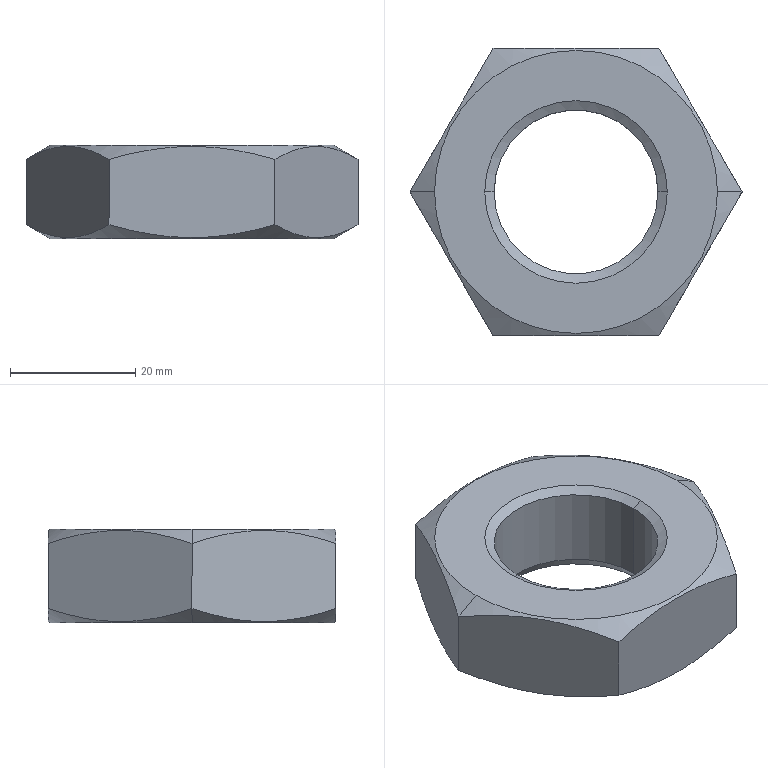Part | SolidWorks | features RevCut 2, Chamfer 1, Extrusion 1, LPattern 1 | 1 solid | 18 faces | box 53.116 x 46 x 15 mm | volume 18987 mm3 | cone 8 | plane 8 | cylinder 2 | commonest cylinder face diameters 26.211 x2
STEP:
#1=CARTESIAN_POINT('',(-13.106,0.,-0.866));
#2=VERTEX_POINT('',#1);
#3=CARTESIAN_POINT('',(13.106,0.,-0.866));
#4=VERTEX_POINT('',#3);
#5=CARTESIAN_POINT('',(0.,0.,-0.866));
#6=DIRECTION('',(0.,0.,1.));
#7=DIRECTION('',(1.,0.,0.));
#8=AXIS2_PLACEMENT_3D('',#5,#6,#7);
#9=CIRCLE('',#8,13.106);
#10=EDGE_CURVE('',#2,#4,#9,.T.);
#11=ORIENTED_EDGE('',*,*,#10,.F.);
#12=CARTESIAN_POINT('',(-14.606,0.,0.));
#13=VERTEX_POINT('',#12);
#14=CARTESIAN_POINT('',(-13.106,0.,-0.866));
#15=DIRECTION('',(-0.866,0.,0.5));
#16=VECTOR('',#15,1000.);
#17=LINE('',#14,#16);
#18=EDGE_CURVE('',#2,#13,#17,.T.);
#19=ORIENTED_EDGE('',*,*,#18,.T.);
#20=CARTESIAN_POINT('',(14.606,0.,0.));
#21=VERTEX_POINT('',#20);
#22=CARTESIAN_POINT('',(0.,0.,0.));
#23=DIRECTION('',(0.,0.,-1.));
#24=DIRECTION('',(1.,0.,0.));
#25=AXIS2_PLACEMENT_3D('',#22,#23,#24);
#26=CIRCLE('',#25,14.606);
#27=EDGE_CURVE('',#21,#13,#26,.T.);
#28=ORIENTED_EDGE('',*,*,#27,.F.);
#29=CARTESIAN_POINT('',(13.106,0.,-0.866));
#30=DIRECTION('',(0.866,0.,0.5));
#31=VECTOR('',#30,1000.);
#32=LINE('',#29,#31);
#33=EDGE_CURVE('',#4,#21,#32,.T.);
#34=ORIENTED_EDGE('',*,*,#33,.F.);
#35=EDGE_LOOP('',(#11,#19,#28,#34));
#36=FACE_OUTER_BOUND('',#35,.T.);
#37=CARTESIAN_POINT('',(0.,0.,-0.866));
#38=DIRECTION('',(0.,0.,1.));
#39=DIRECTION('',(1.,0.,0.));
#40=AXIS2_PLACEMENT_3D('',#37,#38,#39);
#41=CONICAL_SURFACE('',#40,13.106,1.047);
#42=ADVANCED_FACE('',(#36),#41,.F.);
#43=CARTESIAN_POINT('',(13.106,0.,-13.5));
#44=VERTEX_POINT('',#43);
#45=CARTESIAN_POINT('',(-13.106,0.,-13.5));
#46=VERTEX_POINT('',#45);
#47=CARTESIAN_POINT('',(0.,0.,-13.5));
#48=DIRECTION('',(0.,0.,-1.));
#49=DIRECTION('',(1.,0.,0.));
#50=AXIS2_PLACEMENT_3D('',#47,#48,#49);
#51=CIRCLE('',#50,13.106);
#52=EDGE_CURVE('',#44,#46,#51,.T.);
#53=ORIENTED_EDGE('',*,*,#52,.F.);
#54=CARTESIAN_POINT('',(13.972,0.,-15.));
#55=VERTEX_POINT('',#54);
#56=CARTESIAN_POINT('',(13.972,0.,-15.));
#57=DIRECTION('',(0.5,0.,-0.866));
#58=VECTOR('',#57,1000.);
#59=LINE('',#56,#58);
#60=EDGE_CURVE('',#44,#55,#59,.T.);
#61=ORIENTED_EDGE('',*,*,#60,.T.);
#62=CARTESIAN_POINT('',(-13.972,0.,-15.));
#63=VERTEX_POINT('',#62);
#64=CARTESIAN_POINT('',(0.,0.,-15.));
#65=DIRECTION('',(0.,0.,1.));
#66=DIRECTION('',(1.,0.,0.));
#67=AXIS2_PLACEMENT_3D('',#64,#65,#66);
#68=CIRCLE('',#67,13.972);
#69=EDGE_CURVE('',#63,#55,#68,.T.);
#70=ORIENTED_EDGE('',*,*,#69,.F.);
#71=CARTESIAN_POINT('',(-13.972,0.,-15.));
#72=DIRECTION('',(-0.5,0.,-0.866));
#73=VECTOR('',#72,1000.);
#74=LINE('',#71,#73);
#75=EDGE_CURVE('',#46,#63,#74,.T.);
#76=ORIENTED_EDGE('',*,*,#75,.F.);
#77=EDGE_LOOP('',(#53,#61,#70,#76));
#78=FACE_OUTER_BOUND('',#77,.T.);
#79=CARTESIAN_POINT('',(0.,0.,-15.));
#80=DIRECTION('',(0.,0.,-1.));
#81=DIRECTION('',(-1.,0.,0.));
#82=AXIS2_PLACEMENT_3D('',#79,#80,#81);
#83=CONICAL_SURFACE('',#82,13.972,0.5236);
#84=ADVANCED_FACE('',(#78),#83,.F.);
#85=CARTESIAN_POINT('',(-22.625,0.,0.));
#86=VERTEX_POINT('',#85);
#87=CARTESIAN_POINT('',(22.625,0.,0.));
#88=VERTEX_POINT('',#87);
#89=CARTESIAN_POINT('',(0.,0.,0.));
#90=DIRECTION('',(0.,0.,-1.));
#91=DIRECTION('',(-1.,0.,0.));
#92=AXIS2_PLACEMENT_3D('',#89,#90,#91);
#93=CIRCLE('',#92,22.625);
#94=EDGE_CURVE('',#86,#88,#93,.T.);
#95=ORIENTED_EDGE('',*,*,#94,.T.);
#96=CARTESIAN_POINT('',(26.558,0.,-2.271));
#97=VERTEX_POINT('',#96);
#98=CARTESIAN_POINT('',(22.625,0.,0.));
#99=DIRECTION('',(0.866,0.,-0.5));
#100=VECTOR('',#99,1000.);
#101=LINE('',#98,#100);
#102=EDGE_CURVE('',#88,#97,#101,.T.);
#103=ORIENTED_EDGE('',*,*,#102,.T.);
#104=CARTESIAN_POINT('',(13.279,23.,-2.271));
#105=VERTEX_POINT('',#104);
#106=CARTESIAN_POINT('',(26.558,0.,-2.271));
#107=CARTESIAN_POINT('',(25.474,1.878,-1.645));
#108=CARTESIAN_POINT('',(24.382,3.769,-1.129));
#109=CARTESIAN_POINT('',(22.175,7.591,-0.4144));
#110=CARTESIAN_POINT('',(21.06,9.523,-0.218));
#111=CARTESIAN_POINT('',(19.649,11.967,-0.2162));
#112=CARTESIAN_POINT('',(19.365,12.458,-0.2279));
#113=CARTESIAN_POINT('',(18.801,13.436,-0.2751));
#114=CARTESIAN_POINT('',(18.519,13.924,-0.3106));
#115=CARTESIAN_POINT('',(17.678,15.381,-0.4511));
#116=CARTESIAN_POINT('',(17.121,16.346,-0.5901));
#117=CARTESIAN_POINT('',(15.459,19.224,-1.127));
#118=CARTESIAN_POINT('',(14.365,21.12,-1.644));
#119=CARTESIAN_POINT('',(13.279,23.,-2.271));
#120=B_SPLINE_CURVE_WITH_KNOTS('',3,(#106,#107,#108,#109,#110,#111,#112,#113,#114,#115,#116,#117,#118,#119),.UNSPECIFIED.,.F.,.F.,(4,2,2,2,2,2,4),(0.000000238,0.006706,0.01341,0.01509,0.01676,0.02012,0.02682),.UNSPECIFIED.);
#121=EDGE_CURVE('',#97,#105,#120,.T.);
#122=ORIENTED_EDGE('',*,*,#121,.T.);
#123=CARTESIAN_POINT('',(-13.279,23.,-2.271));
#124=VERTEX_POINT('',#123);
#125=CARTESIAN_POINT('',(13.279,23.,-2.271));
#126=CARTESIAN_POINT('',(11.133,23.,-1.651));
#127=CARTESIAN_POINT('',(8.958,23.,-1.135));
#128=CARTESIAN_POINT('',(5.632,23.,-0.595));
#129=CARTESIAN_POINT('',(4.511,23.,-0.4541));
#130=CARTESIAN_POINT('',(2.252,23.,-0.2644));
#131=CARTESIAN_POINT('',(1.126,23.,-0.2166));
#132=CARTESIAN_POINT('',(-2.241,23.,-0.2163));
#133=CARTESIAN_POINT('',(-4.471,23.,-0.409));
#134=CARTESIAN_POINT('',(-7.797,23.,-0.9453));
#135=CARTESIAN_POINT('',(-8.904,23.,-1.165));
#136=CARTESIAN_POINT('',(-11.109,23.,-1.673));
#137=CARTESIAN_POINT('',(-12.199,23.,-1.959));
#138=CARTESIAN_POINT('',(-13.279,23.,-2.271));
#139=B_SPLINE_CURVE_WITH_KNOTS('',3,(#125,#126,#127,#128,#129,#130,#131,#132,#133,#134,#135,#136,#137,#138),.UNSPECIFIED.,.F.,.F.,(4,2,2,2,2,2,4),(0.00977,0.01647,0.01982,0.02317,0.02987,0.03323,0.03658),.UNSPECIFIED.);
#140=EDGE_CURVE('',#105,#124,#139,.T.);
#141=ORIENTED_EDGE('',*,*,#140,.T.);
#142=CARTESIAN_POINT('',(-26.558,0.,-2.271));
#143=VERTEX_POINT('',#142);
#144=CARTESIAN_POINT('',(-13.279,23.,-2.271));
#145=CARTESIAN_POINT('',(-14.363,21.122,-1.645));
#146=CARTESIAN_POINT('',(-15.455,19.231,-1.129));
#147=CARTESIAN_POINT('',(-17.662,15.409,-0.4144));
#148=CARTESIAN_POINT('',(-18.777,13.477,-0.218));
#149=CARTESIAN_POINT('',(-20.188,11.033,-0.2162));
#150=CARTESIAN_POINT('',(-20.472,10.542,-0.2279));
#151=CARTESIAN_POINT('',(-21.037,9.564,-0.2751));
#152=CARTESIAN_POINT('',(-21.318,9.076,-0.3106));
#153=CARTESIAN_POINT('',(-22.159,7.619,-0.4511));
#154=CARTESIAN_POINT('',(-22.717,6.654,-0.5901));
#155=CARTESIAN_POINT('',(-24.378,3.776,-1.127));
#156=CARTESIAN_POINT('',(-25.473,1.88,-1.644));
#157=CARTESIAN_POINT('',(-26.558,0.,-2.271));
#158=B_SPLINE_CURVE_WITH_KNOTS('',3,(#144,#145,#146,#147,#148,#149,#150,#151,#152,#153,#154,#155,#156,#157),.UNSPECIFIED.,.F.,.F.,(4,2,2,2,2,2,4),(0.000000238,0.006706,0.01341,0.01509,0.01676,0.02012,0.02682),.UNSPECIFIED.);
#159=EDGE_CURVE('',#124,#143,#158,.T.);
#160=ORIENTED_EDGE('',*,*,#159,.T.);
#161=CARTESIAN_POINT('',(-22.625,0.,0.));
#162=DIRECTION('',(-0.866,0.,-0.5));
#163=VECTOR('',#162,1000.);
#164=LINE('',#161,#163);
#165=EDGE_CURVE('',#86,#143,#164,.T.);
#166=ORIENTED_EDGE('',*,*,#165,.F.);
#167=EDGE_LOOP('',(#95,#103,#122,#141,#160,#166));
#168=FACE_OUTER_BOUND('',#167,.T.);
#169=CARTESIAN_POINT('',(0.,0.,0.));
#170=DIRECTION('',(0.,0.,-1.));
#171=DIRECTION('',(-1.,0.,0.));
#172=AXIS2_PLACEMENT_3D('',#169,#170,#171);
#173=CONICAL_SURFACE('',#172,22.625,1.047);
#174=ADVANCED_FACE('',(#168),#173,.T.);
#175=CARTESIAN_POINT('',(-22.625,0.,-15.));
#176=VERTEX_POINT('',#175);
#177=CARTESIAN_POINT('',(22.625,0.,-15.));
#178=VERTEX_POINT('',#177);
#179=CARTESIAN_POINT('',(0.,0.,-15.));
#180=DIRECTION('',(0.,0.,-1.));
#181=DIRECTION('',(-1.,0.,0.));
#182=AXIS2_PLACEMENT_3D('',#179,#180,#181);
#183=CIRCLE('',#182,22.625);
#184=EDGE_CURVE('',#176,#178,#183,.T.);
#185=ORIENTED_EDGE('',*,*,#184,.F.);
#186=CARTESIAN_POINT('',(-26.558,0.,-12.729));
#187=VERTEX_POINT('',#186);
#188=CARTESIAN_POINT('',(-26.558,0.,-12.729));
#189=DIRECTION('',(-0.866,0.,0.5));
#190=VECTOR('',#189,1000.);
#191=LINE('',#188,#190);
#192=EDGE_CURVE('',#176,#187,#191,.T.);
#193=ORIENTED_EDGE('',*,*,#192,.T.);
#194=CARTESIAN_POINT('',(-13.279,23.,-12.729));
#195=VERTEX_POINT('',#194);
#196=CARTESIAN_POINT('',(-26.558,0.,-12.729));
#197=CARTESIAN_POINT('',(-25.474,1.878,-13.355));
#198=CARTESIAN_POINT('',(-24.382,3.769,-13.871));
#199=CARTESIAN_POINT('',(-22.175,7.591,-14.586));
#200=CARTESIAN_POINT('',(-21.06,9.523,-14.782));
#201=CARTESIAN_POINT('',(-19.649,11.967,-14.784));
#202=CARTESIAN_POINT('',(-19.365,12.458,-14.772));
#203=CARTESIAN_POINT('',(-18.801,13.436,-14.725));
#204=CARTESIAN_POINT('',(-18.519,13.924,-14.689));
#205=CARTESIAN_POINT('',(-17.678,15.381,-14.549));
#206=CARTESIAN_POINT('',(-17.121,16.346,-14.41));
#207=CARTESIAN_POINT('',(-15.459,19.224,-13.873));
#208=CARTESIAN_POINT('',(-14.365,21.12,-13.356));
#209=CARTESIAN_POINT('',(-13.279,23.,-12.729));
#210=B_SPLINE_CURVE_WITH_KNOTS('',3,(#196,#197,#198,#199,#200,#201,#202,#203,#204,#205,#206,#207,#208,#209),.UNSPECIFIED.,.F.,.F.,(4,2,2,2,2,2,4),(0.000000238,0.006706,0.01341,0.01509,0.01676,0.02012,0.02682),.UNSPECIFIED.);
#211=EDGE_CURVE('',#187,#195,#210,.T.);
#212=ORIENTED_EDGE('',*,*,#211,.T.);
#213=CARTESIAN_POINT('',(13.279,23.,-12.729));
#214=VERTEX_POINT('',#213);
#215=CARTESIAN_POINT('',(-13.279,23.,-12.729));
#216=CARTESIAN_POINT('',(-12.199,23.,-13.041));
#217=CARTESIAN_POINT('',(-11.109,23.,-13.327));
#218=CARTESIAN_POINT('',(-8.904,23.,-13.835));
#219=CARTESIAN_POINT('',(-7.797,23.,-14.055));
#220=CARTESIAN_POINT('',(-4.471,23.,-14.591));
#221=CARTESIAN_POINT('',(-2.241,23.,-14.784));
#222=CARTESIAN_POINT('',(1.126,23.,-14.783));
#223=CARTESIAN_POINT('',(2.252,23.,-14.736));
#224=CARTESIAN_POINT('',(4.511,23.,-14.546));
#225=CARTESIAN_POINT('',(5.632,23.,-14.405));
#226=CARTESIAN_POINT('',(8.958,23.,-13.865));
#227=CARTESIAN_POINT('',(11.133,23.,-13.349));
#228=CARTESIAN_POINT('',(13.279,23.,-12.729));
#229=B_SPLINE_CURVE_WITH_KNOTS('',3,(#215,#216,#217,#218,#219,#220,#221,#222,#223,#224,#225,#226,#227,#228),.UNSPECIFIED.,.F.,.F.,(4,2,2,2,2,2,4),(0.02366,0.02702,0.03038,0.0371,0.04045,0.04381,0.05053),.UNSPECIFIED.);
#230=EDGE_CURVE('',#195,#214,#229,.T.);
#231=ORIENTED_EDGE('',*,*,#230,.T.);
#232=CARTESIAN_POINT('',(26.558,0.,-12.729));
#233=VERTEX_POINT('',#232);
#234=CARTESIAN_POINT('',(13.279,23.,-12.729));
#235=CARTESIAN_POINT('',(14.363,21.122,-13.355));
#236=CARTESIAN_POINT('',(15.455,19.231,-13.871));
#237=CARTESIAN_POINT('',(17.662,15.409,-14.586));
#238=CARTESIAN_POINT('',(18.777,13.477,-14.782));
#239=CARTESIAN_POINT('',(20.188,11.033,-14.784));
#240=CARTESIAN_POINT('',(20.472,10.542,-14.772));
#241=CARTESIAN_POINT('',(21.037,9.564,-14.725));
#242=CARTESIAN_POINT('',(21.318,9.076,-14.689));
#243=CARTESIAN_POINT('',(22.159,7.619,-14.549));
#244=CARTESIAN_POINT('',(22.717,6.654,-14.41));
#245=CARTESIAN_POINT('',(24.378,3.776,-13.873));
#246=CARTESIAN_POINT('',(25.473,1.88,-13.356));
#247=CARTESIAN_POINT('',(26.558,0.,-12.729));
#248=B_SPLINE_CURVE_WITH_KNOTS('',3,(#234,#235,#236,#237,#238,#239,#240,#241,#242,#243,#244,#245,#246,#247),.UNSPECIFIED.,.F.,.F.,(4,2,2,2,2,2,4),(0.000000238,0.006706,0.01341,0.01509,0.01676,0.02012,0.02682),.UNSPECIFIED.);
#249=EDGE_CURVE('',#214,#233,#248,.T.);
#250=ORIENTED_EDGE('',*,*,#249,.T.);
#251=CARTESIAN_POINT('',(26.558,0.,-12.729));
#252=DIRECTION('',(0.866,0.,0.5));
#253=VECTOR('',#252,1000.);
#254=LINE('',#251,#253);
#255=EDGE_CURVE('',#178,#233,#254,.T.);
#256=ORIENTED_EDGE('',*,*,#255,.F.);
#257=EDGE_LOOP('',(#185,#193,#212,#231,#250,#256));
#258=FACE_OUTER_BOUND('',#257,.T.);
#259=CARTESIAN_POINT('',(0.,0.,-12.729));
#260=DIRECTION('',(0.,0.,1.));
#261=DIRECTION('',(1.,0.,0.));
#262=AXIS2_PLACEMENT_3D('',#259,#260,#261);
#263=CONICAL_SURFACE('',#262,26.558,1.047);
#264=ADVANCED_FACE('',(#258),#263,.T.);
#265=ORIENTED_EDGE('',*,*,#52,.T.);
#266=CARTESIAN_POINT('',(-13.106,0.,-15.));
#267=DIRECTION('',(0.,0.,1.));
#268=VECTOR('',#267,1000.);
#269=LINE('',#266,#268);
#270=EDGE_CURVE('',#46,#2,#269,.T.);
#271=ORIENTED_EDGE('',*,*,#270,.T.);
#272=ORIENTED_EDGE('',*,*,#10,.T.);
#273=CARTESIAN_POINT('',(13.106,0.,-15.));
#274=DIRECTION('',(0.,0.,1.));
#275=VECTOR('',#274,1000.);
#276=LINE('',#273,#275);
#277=EDGE_CURVE('',#44,#4,#276,.T.);
#278=ORIENTED_EDGE('',*,*,#277,.F.);
#279=EDGE_LOOP('',(#265,#271,#272,#278));
#280=FACE_OUTER_BOUND('',#279,.T.);
#281=CARTESIAN_POINT('',(0.,0.,-15.));
#282=DIRECTION('',(0.,0.,1.));
#283=DIRECTION('',(1.,0.,0.));
#284=AXIS2_PLACEMENT_3D('',#281,#282,#283);
#285=CYLINDRICAL_SURFACE('',#284,13.106);
#286=ADVANCED_FACE('',(#280),#285,.F.);
#287=CARTESIAN_POINT('',(-13.279,-23.,-2.271));
#288=VERTEX_POINT('',#287);
#289=CARTESIAN_POINT('',(13.279,-23.,-2.271));
#290=VERTEX_POINT('',#289);
#291=CARTESIAN_POINT('',(-13.279,-23.,-2.271));
#292=CARTESIAN_POINT('',(-12.199,-23.,-1.959));
#293=CARTESIAN_POINT('',(-11.109,-23.,-1.673));
#294=CARTESIAN_POINT('',(-8.904,-23.,-1.165));
#295=CARTESIAN_POINT('',(-7.797,-23.,-0.9453));
#296=CARTESIAN_POINT('',(-4.471,-23.,-0.409));
#297=CARTESIAN_POINT('',(-2.241,-23.,-0.2163));
#298=CARTESIAN_POINT('',(1.126,-23.,-0.2166));
#299=CARTESIAN_POINT('',(2.252,-23.,-0.2644));
#300=CARTESIAN_POINT('',(4.511,-23.,-0.4541));
#301=CARTESIAN_POINT('',(5.632,-23.,-0.595));
#302=CARTESIAN_POINT('',(8.958,-23.,-1.135));
#303=CARTESIAN_POINT('',(11.133,-23.,-1.651));
#304=CARTESIAN_POINT('',(13.279,-23.,-2.271));
#305=B_SPLINE_CURVE_WITH_KNOTS('',3,(#291,#292,#293,#294,#295,#296,#297,#298,#299,#300,#301,#302,#303,#304),.UNSPECIFIED.,.F.,.F.,(4,2,2,2,2,2,4),(0.02366,0.02702,0.03038,0.0371,0.04045,0.04381,0.05053),.UNSPECIFIED.);
#306=EDGE_CURVE('',#288,#290,#305,.T.);
#307=ORIENTED_EDGE('',*,*,#306,.F.);
#308=CARTESIAN_POINT('',(-13.279,-23.,-12.729));
#309=VERTEX_POINT('',#308);
#310=CARTESIAN_POINT('',(-13.279,-23.,-15.));
#311=DIRECTION('',(0.,0.,1.));
#312=VECTOR('',#311,1000.);
#313=LINE('',#310,#312);
#314=EDGE_CURVE('',#309,#288,#313,.T.);
#315=ORIENTED_EDGE('',*,*,#314,.F.);
#316=CARTESIAN_POINT('',(13.279,-23.,-12.729));
#317=VERTEX_POINT('',#316);
#318=CARTESIAN_POINT('',(13.279,-23.,-12.729));
#319=CARTESIAN_POINT('',(11.133,-23.,-13.349));
#320=CARTESIAN_POINT('',(8.958,-23.,-13.865));
#321=CARTESIAN_POINT('',(5.632,-23.,-14.405));
#322=CARTESIAN_POINT('',(4.511,-23.,-14.546));
#323=CARTESIAN_POINT('',(2.252,-23.,-14.736));
#324=CARTESIAN_POINT('',(1.126,-23.,-14.783));
#325=CARTESIAN_POINT('',(-2.241,-23.,-14.784));
#326=CARTESIAN_POINT('',(-4.471,-23.,-14.591));
#327=CARTESIAN_POINT('',(-7.797,-23.,-14.055));
#328=CARTESIAN_POINT('',(-8.904,-23.,-13.835));
#329=CARTESIAN_POINT('',(-11.109,-23.,-13.327));
#330=CARTESIAN_POINT('',(-12.199,-23.,-13.041));
#331=CARTESIAN_POINT('',(-13.279,-23.,-12.729));
#332=B_SPLINE_CURVE_WITH_KNOTS('',3,(#318,#319,#320,#321,#322,#323,#324,#325,#326,#327,#328,#329,#330,#331),.UNSPECIFIED.,.F.,.F.,(4,2,2,2,2,2,4),(0.00977,0.01647,0.01982,0.02317,0.02987,0.03323,0.03658),.UNSPECIFIED.);
#333=EDGE_CURVE('',#317,#309,#332,.T.);
#334=ORIENTED_EDGE('',*,*,#333,.F.);
#335=CARTESIAN_POINT('',(13.279,-23.,-15.));
#336=DIRECTION('',(0.,0.,1.));
#337=VECTOR('',#336,1000.);
#338=LINE('',#335,#337);
#339=EDGE_CURVE('',#317,#290,#338,.T.);
#340=ORIENTED_EDGE('',*,*,#339,.T.);
#341=EDGE_LOOP('',(#307,#315,#334,#340));
#342=FACE_OUTER_BOUND('',#341,.T.);
#343=CARTESIAN_POINT('',(-13.279,-23.,-15.));
#344=DIRECTION('',(0.,-1.,0.));
#345=DIRECTION('',(1.,0.,0.));
#346=AXIS2_PLACEMENT_3D('',#343,#344,#345);
#347=PLANE('',#346);
#348=ADVANCED_FACE('',(#342),#347,.T.);
#349=CARTESIAN_POINT('',(-26.558,0.,-2.271));
#350=CARTESIAN_POINT('',(-25.474,-1.878,-1.645));
#351=CARTESIAN_POINT('',(-24.382,-3.769,-1.129));
#352=CARTESIAN_POINT('',(-22.175,-7.591,-0.4144));
#353=CARTESIAN_POINT('',(-21.06,-9.523,-0.218));
#354=CARTESIAN_POINT('',(-19.649,-11.967,-0.2162));
#355=CARTESIAN_POINT('',(-19.365,-12.458,-0.2279));
#356=CARTESIAN_POINT('',(-18.801,-13.436,-0.2751));
#357=CARTESIAN_POINT('',(-18.519,-13.924,-0.3106));
#358=CARTESIAN_POINT('',(-17.678,-15.381,-0.4511));
#359=CARTESIAN_POINT('',(-17.121,-16.346,-0.5901));
#360=CARTESIAN_POINT('',(-15.459,-19.224,-1.127));
#361=CARTESIAN_POINT('',(-14.365,-21.12,-1.644));
#362=CARTESIAN_POINT('',(-13.279,-23.,-2.271));
#363=B_SPLINE_CURVE_WITH_KNOTS('',3,(#349,#350,#351,#352,#353,#354,#355,#356,#357,#358,#359,#360,#361,#362),.UNSPECIFIED.,.F.,.F.,(4,2,2,2,2,2,4),(0.000000238,0.006706,0.01341,0.01509,0.01676,0.02012,0.02682),.UNSPECIFIED.);
#364=EDGE_CURVE('',#143,#288,#363,.T.);
#365=ORIENTED_EDGE('',*,*,#364,.F.);
#366=CARTESIAN_POINT('',(-26.558,0.,-15.));
#367=DIRECTION('',(0.,0.,1.));
#368=VECTOR('',#367,1000.);
#369=LINE('',#366,#368);
#370=EDGE_CURVE('',#187,#143,#369,.T.);
#371=ORIENTED_EDGE('',*,*,#370,.F.);
#372=CARTESIAN_POINT('',(-13.279,-23.,-12.729));
#373=CARTESIAN_POINT('',(-14.363,-21.122,-13.355));
#374=CARTESIAN_POINT('',(-15.455,-19.231,-13.871));
#375=CARTESIAN_POINT('',(-17.662,-15.409,-14.586));
#376=CARTESIAN_POINT('',(-18.777,-13.477,-14.782));
#377=CARTESIAN_POINT('',(-20.188,-11.033,-14.784));
#378=CARTESIAN_POINT('',(-20.472,-10.542,-14.772));
#379=CARTESIAN_POINT('',(-21.037,-9.564,-14.725));
#380=CARTESIAN_POINT('',(-21.318,-9.076,-14.689));
#381=CARTESIAN_POINT('',(-22.159,-7.619,-14.549));
#382=CARTESIAN_POINT('',(-22.717,-6.654,-14.41));
#383=CARTESIAN_POINT('',(-24.378,-3.776,-13.873));
#384=CARTESIAN_POINT('',(-25.473,-1.88,-13.356));
#385=CARTESIAN_POINT('',(-26.558,0.,-12.729));
#386=B_SPLINE_CURVE_WITH_KNOTS('',3,(#372,#373,#374,#375,#376,#377,#378,#379,#380,#381,#382,#383,#384,#385),.UNSPECIFIED.,.F.,.F.,(4,2,2,2,2,2,4),(0.000000238,0.006706,0.01341,0.01509,0.01676,0.02012,0.02682),.UNSPECIFIED.);
#387=EDGE_CURVE('',#309,#187,#386,.T.);
#388=ORIENTED_EDGE('',*,*,#387,.F.);
#389=ORIENTED_EDGE('',*,*,#314,.T.);
#390=EDGE_LOOP('',(#365,#371,#388,#389));
#391=FACE_OUTER_BOUND('',#390,.T.);
#392=CARTESIAN_POINT('',(-26.558,0.,-15.));
#393=DIRECTION('',(-0.866,-0.5,0.));
#394=DIRECTION('',(0.5,-0.866,0.));
#395=AXIS2_PLACEMENT_3D('',#392,#393,#394);
#396=PLANE('',#395);
#397=ADVANCED_FACE('',(#391),#396,.T.);
#398=ORIENTED_EDGE('',*,*,#159,.F.);
#399=CARTESIAN_POINT('',(-13.279,23.,-15.));
#400=DIRECTION('',(0.,0.,1.));
#401=VECTOR('',#400,1000.);
#402=LINE('',#399,#401);
#403=EDGE_CURVE('',#195,#124,#402,.T.);
#404=ORIENTED_EDGE('',*,*,#403,.F.);
#405=ORIENTED_EDGE('',*,*,#211,.F.);
#406=ORIENTED_EDGE('',*,*,#370,.T.);
#407=EDGE_LOOP('',(#398,#404,#405,#406));
#408=FACE_OUTER_BOUND('',#407,.T.);
#409=CARTESIAN_POINT('',(-13.279,23.,-15.));
#410=DIRECTION('',(-0.866,0.5,0.));
#411=DIRECTION('',(-0.5,-0.866,0.));
#412=AXIS2_PLACEMENT_3D('',#409,#410,#411);
#413=PLANE('',#412);
#414=ADVANCED_FACE('',(#408),#413,.T.);
#415=ORIENTED_EDGE('',*,*,#140,.F.);
#416=CARTESIAN_POINT('',(13.279,23.,-15.));
#417=DIRECTION('',(0.,0.,1.));
#418=VECTOR('',#417,1000.);
#419=LINE('',#416,#418);
#420=EDGE_CURVE('',#214,#105,#419,.T.);
#421=ORIENTED_EDGE('',*,*,#420,.F.);
#422=ORIENTED_EDGE('',*,*,#230,.F.);
#423=ORIENTED_EDGE('',*,*,#403,.T.);
#424=EDGE_LOOP('',(#415,#421,#422,#423));
#425=FACE_OUTER_BOUND('',#424,.T.);
#426=CARTESIAN_POINT('',(13.279,23.,-15.));
#427=DIRECTION('',(0.,1.,0.));
#428=DIRECTION('',(0.,0.,1.));
#429=AXIS2_PLACEMENT_3D('',#426,#427,#428);
#430=PLANE('',#429);
#431=ADVANCED_FACE('',(#425),#430,.T.);
#432=ORIENTED_EDGE('',*,*,#121,.F.);
#433=CARTESIAN_POINT('',(26.558,0.,-15.));
#434=DIRECTION('',(0.,0.,1.));
#435=VECTOR('',#434,1000.);
#436=LINE('',#433,#435);
#437=EDGE_CURVE('',#233,#97,#436,.T.);
#438=ORIENTED_EDGE('',*,*,#437,.F.);
#439=ORIENTED_EDGE('',*,*,#249,.F.);
#440=ORIENTED_EDGE('',*,*,#420,.T.);
#441=EDGE_LOOP('',(#432,#438,#439,#440));
#442=FACE_OUTER_BOUND('',#441,.T.);
#443=CARTESIAN_POINT('',(26.558,0.,-15.));
#444=DIRECTION('',(0.866,0.5,0.));
#445=DIRECTION('',(-0.5,0.866,0.));
#446=AXIS2_PLACEMENT_3D('',#443,#444,#445);
#447=PLANE('',#446);
#448=ADVANCED_FACE('',(#442),#447,.T.);
#449=CARTESIAN_POINT('',(13.279,-23.,-2.271));
#450=CARTESIAN_POINT('',(14.363,-21.122,-1.645));
#451=CARTESIAN_POINT('',(15.455,-19.231,-1.129));
#452=CARTESIAN_POINT('',(17.662,-15.409,-0.4144));
#453=CARTESIAN_POINT('',(18.777,-13.477,-0.218));
#454=CARTESIAN_POINT('',(20.188,-11.033,-0.2162));
#455=CARTESIAN_POINT('',(20.472,-10.542,-0.2279));
#456=CARTESIAN_POINT('',(21.037,-9.564,-0.2751));
#457=CARTESIAN_POINT('',(21.318,-9.076,-0.3106));
#458=CARTESIAN_POINT('',(22.159,-7.619,-0.4511));
#459=CARTESIAN_POINT('',(22.717,-6.654,-0.5901));
#460=CARTESIAN_POINT('',(24.378,-3.776,-1.127));
#461=CARTESIAN_POINT('',(25.473,-1.88,-1.644));
#462=CARTESIAN_POINT('',(26.558,0.,-2.271));
#463=B_SPLINE_CURVE_WITH_KNOTS('',3,(#449,#450,#451,#452,#453,#454,#455,#456,#457,#458,#459,#460,#461,#462),.UNSPECIFIED.,.F.,.F.,(4,2,2,2,2,2,4),(0.000000238,0.006706,0.01341,0.01509,0.01676,0.02012,0.02682),.UNSPECIFIED.);
#464=EDGE_CURVE('',#290,#97,#463,.T.);
#465=ORIENTED_EDGE('',*,*,#464,.F.);
#466=ORIENTED_EDGE('',*,*,#339,.F.);
#467=CARTESIAN_POINT('',(26.558,0.,-12.729));
#468=CARTESIAN_POINT('',(25.474,-1.878,-13.355));
#469=CARTESIAN_POINT('',(24.382,-3.769,-13.871));
#470=CARTESIAN_POINT('',(22.175,-7.591,-14.586));
#471=CARTESIAN_POINT('',(21.06,-9.523,-14.782));
#472=CARTESIAN_POINT('',(19.649,-11.967,-14.784));
#473=CARTESIAN_POINT('',(19.365,-12.458,-14.772));
#474=CARTESIAN_POINT('',(18.801,-13.436,-14.725));
#475=CARTESIAN_POINT('',(18.519,-13.924,-14.689));
#476=CARTESIAN_POINT('',(17.678,-15.381,-14.549));
#477=CARTESIAN_POINT('',(17.121,-16.346,-14.41));
#478=CARTESIAN_POINT('',(15.459,-19.224,-13.873));
#479=CARTESIAN_POINT('',(14.365,-21.12,-13.356));
#480=CARTESIAN_POINT('',(13.279,-23.,-12.729));
#481=B_SPLINE_CURVE_WITH_KNOTS('',3,(#467,#468,#469,#470,#471,#472,#473,#474,#475,#476,#477,#478,#479,#480),.UNSPECIFIED.,.F.,.F.,(4,2,2,2,2,2,4),(0.000000238,0.006706,0.01341,0.01509,0.01676,0.02012,0.02682),.UNSPECIFIED.);
#482=EDGE_CURVE('',#233,#317,#481,.T.);
#483=ORIENTED_EDGE('',*,*,#482,.F.);
#484=ORIENTED_EDGE('',*,*,#437,.T.);
#485=EDGE_LOOP('',(#465,#466,#483,#484));
#486=FACE_OUTER_BOUND('',#485,.T.);
#487=CARTESIAN_POINT('',(13.279,-23.,-15.));
#488=DIRECTION('',(0.866,-0.5,0.));
#489=DIRECTION('',(0.5,0.866,0.));
#490=AXIS2_PLACEMENT_3D('',#487,#488,#489);
#491=PLANE('',#490);
#492=ADVANCED_FACE('',(#486),#491,.T.);
#493=ORIENTED_EDGE('',*,*,#69,.T.);
#494=CARTESIAN_POINT('',(0.,0.,-15.));
#495=DIRECTION('',(0.,0.,1.));
#496=DIRECTION('',(1.,0.,0.));
#497=AXIS2_PLACEMENT_3D('',#494,#495,#496);
#498=CIRCLE('',#497,13.972);
#499=EDGE_CURVE('',#55,#63,#498,.T.);
#500=ORIENTED_EDGE('',*,*,#499,.T.);
#501=EDGE_LOOP('',(#493,#500));
#502=FACE_BOUND('',#501,.T.);
#503=CARTESIAN_POINT('',(0.,0.,-15.));
#504=DIRECTION('',(0.,0.,-1.));
#505=DIRECTION('',(-1.,0.,0.));
#506=AXIS2_PLACEMENT_3D('',#503,#504,#505);
#507=CIRCLE('',#506,22.625);
#508=EDGE_CURVE('',#178,#176,#507,.T.);
#509=ORIENTED_EDGE('',*,*,#508,.T.);
#510=ORIENTED_EDGE('',*,*,#184,.T.);
#511=EDGE_LOOP('',(#509,#510));
#512=FACE_OUTER_BOUND('',#511,.T.);
#513=CARTESIAN_POINT('',(13.279,-23.,-15.));
#514=DIRECTION('',(0.,0.,1.));
#515=DIRECTION('',(1.,0.,0.));
#516=AXIS2_PLACEMENT_3D('',#513,#514,#515);
#517=PLANE('',#516);
#518=ADVANCED_FACE('',(#502,#512),#517,.F.);
#519=ORIENTED_EDGE('',*,*,#27,.T.);
#520=CARTESIAN_POINT('',(0.,0.,0.));
#521=DIRECTION('',(0.,0.,-1.));
#522=DIRECTION('',(1.,0.,0.));
#523=AXIS2_PLACEMENT_3D('',#520,#521,#522);
#524=CIRCLE('',#523,14.606);
#525=EDGE_CURVE('',#13,#21,#524,.T.);
#526=ORIENTED_EDGE('',*,*,#525,.T.);
#527=EDGE_LOOP('',(#519,#526));
#528=FACE_BOUND('',#527,.T.);
#529=ORIENTED_EDGE('',*,*,#94,.F.);
#530=CARTESIAN_POINT('',(0.,0.,0.));
#531=DIRECTION('',(0.,0.,-1.));
#532=DIRECTION('',(-1.,0.,0.));
#533=AXIS2_PLACEMENT_3D('',#530,#531,#532);
#534=CIRCLE('',#533,22.625);
#535=EDGE_CURVE('',#88,#86,#534,.T.);
#536=ORIENTED_EDGE('',*,*,#535,.F.);
#537=EDGE_LOOP('',(#529,#536));
#538=FACE_OUTER_BOUND('',#537,.T.);
#539=CARTESIAN_POINT('',(13.279,-23.,0.));
#540=DIRECTION('',(0.,0.,1.));
#541=DIRECTION('',(1.,0.,0.));
#542=AXIS2_PLACEMENT_3D('',#539,#540,#541);
#543=PLANE('',#542);
#544=ADVANCED_FACE('',(#528,#538),#543,.T.);
#545=ORIENTED_EDGE('',*,*,#270,.F.);
#546=CARTESIAN_POINT('',(0.,0.,-13.5));
#547=DIRECTION('',(0.,0.,-1.));
#548=DIRECTION('',(1.,0.,0.));
#549=AXIS2_PLACEMENT_3D('',#546,#547,#548);
#550=CIRCLE('',#549,13.106);
#551=EDGE_CURVE('',#46,#44,#550,.T.);
#552=ORIENTED_EDGE('',*,*,#551,.T.);
#553=ORIENTED_EDGE('',*,*,#277,.T.);
#554=CARTESIAN_POINT('',(0.,0.,-0.866));
#555=DIRECTION('',(0.,0.,1.));
#556=DIRECTION('',(1.,0.,0.));
#557=AXIS2_PLACEMENT_3D('',#554,#555,#556);
#558=CIRCLE('',#557,13.106);
#559=EDGE_CURVE('',#4,#2,#558,.T.);
#560=ORIENTED_EDGE('',*,*,#559,.T.);
#561=EDGE_LOOP('',(#545,#552,#553,#560));
#562=FACE_OUTER_BOUND('',#561,.T.);
#563=CARTESIAN_POINT('',(0.,0.,-15.));
#564=DIRECTION('',(0.,0.,1.));
#565=DIRECTION('',(1.,0.,0.));
#566=AXIS2_PLACEMENT_3D('',#563,#564,#565);
#567=CYLINDRICAL_SURFACE('',#566,13.106);
#568=ADVANCED_FACE('',(#562),#567,.F.);
#569=ORIENTED_EDGE('',*,*,#192,.F.);
#570=ORIENTED_EDGE('',*,*,#508,.F.);
#571=ORIENTED_EDGE('',*,*,#255,.T.);
#572=ORIENTED_EDGE('',*,*,#482,.T.);
#573=ORIENTED_EDGE('',*,*,#333,.T.);
#574=ORIENTED_EDGE('',*,*,#387,.T.);
#575=EDGE_LOOP('',(#569,#570,#571,#572,#573,#574));
#576=FACE_OUTER_BOUND('',#575,.T.);
#577=CARTESIAN_POINT('',(0.,0.,-12.729));
#578=DIRECTION('',(0.,0.,1.));
#579=DIRECTION('',(1.,0.,0.));
#580=AXIS2_PLACEMENT_3D('',#577,#578,#579);
#581=CONICAL_SURFACE('',#580,26.558,1.047);
#582=ADVANCED_FACE('',(#576),#581,.T.);
#583=ORIENTED_EDGE('',*,*,#102,.F.);
#584=ORIENTED_EDGE('',*,*,#535,.T.);
#585=ORIENTED_EDGE('',*,*,#165,.T.);
#586=ORIENTED_EDGE('',*,*,#364,.T.);
#587=ORIENTED_EDGE('',*,*,#306,.T.);
#588=ORIENTED_EDGE('',*,*,#464,.T.);
#589=EDGE_LOOP('',(#583,#584,#585,#586,#587,#588));
#590=FACE_OUTER_BOUND('',#589,.T.);
#591=CARTESIAN_POINT('',(0.,0.,0.));
#592=DIRECTION('',(0.,0.,-1.));
#593=DIRECTION('',(-1.,0.,0.));
#594=AXIS2_PLACEMENT_3D('',#591,#592,#593);
#595=CONICAL_SURFACE('',#594,22.625,1.047);
#596=ADVANCED_FACE('',(#590),#595,.T.);
#597=ORIENTED_EDGE('',*,*,#60,.F.);
#598=ORIENTED_EDGE('',*,*,#551,.F.);
#599=ORIENTED_EDGE('',*,*,#75,.T.);
#600=ORIENTED_EDGE('',*,*,#499,.F.);
#601=EDGE_LOOP('',(#597,#598,#599,#600));
#602=FACE_OUTER_BOUND('',#601,.T.);
#603=CARTESIAN_POINT('',(0.,0.,-15.));
#604=DIRECTION('',(0.,0.,-1.));
#605=DIRECTION('',(-1.,0.,0.));
#606=AXIS2_PLACEMENT_3D('',#603,#604,#605);
#607=CONICAL_SURFACE('',#606,13.972,0.5236);
#608=ADVANCED_FACE('',(#602),#607,.F.);
#609=ORIENTED_EDGE('',*,*,#18,.F.);
#610=ORIENTED_EDGE('',*,*,#559,.F.);
#611=ORIENTED_EDGE('',*,*,#33,.T.);
#612=ORIENTED_EDGE('',*,*,#525,.F.);
#613=EDGE_LOOP('',(#609,#610,#611,#612));
#614=FACE_OUTER_BOUND('',#613,.T.);
#615=CARTESIAN_POINT('',(0.,0.,-0.866));
#616=DIRECTION('',(0.,0.,1.));
#617=DIRECTION('',(1.,0.,0.));
#618=AXIS2_PLACEMENT_3D('',#615,#616,#617);
#619=CONICAL_SURFACE('',#618,13.106,1.047);
#620=ADVANCED_FACE('',(#614),#619,.F.);
#621=CLOSED_SHELL('',(#42,#84,#174,#264,#286,#348,#397,#414,#431,#448,#492,#518,#544,#568,#582,#596,#608,#620));
#622=MANIFOLD_SOLID_BREP('',#621);
#623=CARTESIAN_POINT('',(0.,0.,0.));
#624=DIRECTION('',(0.,0.,1.));
#625=DIRECTION('',(1.,0.,0.));
#626=AXIS2_PLACEMENT_3D('',#623,#624,#625);
#627=(LENGTH_UNIT()NAMED_UNIT(*)SI_UNIT(.MILLI.,.METRE.));
#628=UNCERTAINTY_MEASURE_WITH_UNIT(LENGTH_MEASURE(0.00001),#627,'','');
#629=(NAMED_UNIT(*)PLANE_ANGLE_UNIT()SI_UNIT($,.RADIAN.));
#630=(NAMED_UNIT(*)SI_UNIT($,.STERADIAN.)SOLID_ANGLE_UNIT());
#631=(GEOMETRIC_REPRESENTATION_CONTEXT(3)GLOBAL_UNCERTAINTY_ASSIGNED_CONTEXT((#628))GLOBAL_UNIT_ASSIGNED_CONTEXT((#627,#629,#630))REPRESENTATION_CONTEXT('',''));
#632=ADVANCED_BREP_SHAPE_REPRESENTATION('',(#622,#626),#631);